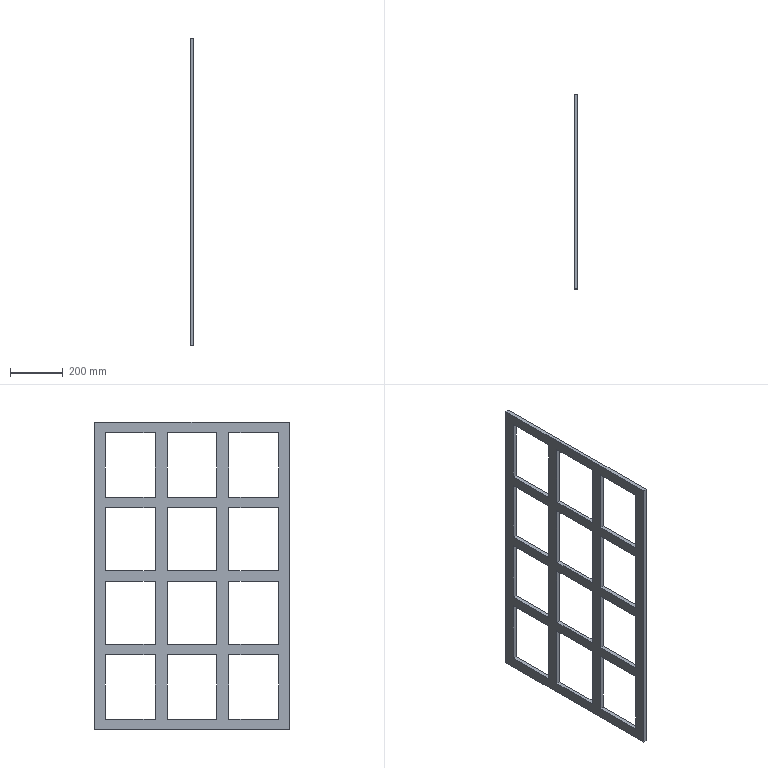Part | SolidWorks | features Extrusion 1, ICE 1, MirrorPattern 1 | 1 solid | 54 faces | box 15 x 740 x 1170 mm | volume 4693500 mm3 | plane 54